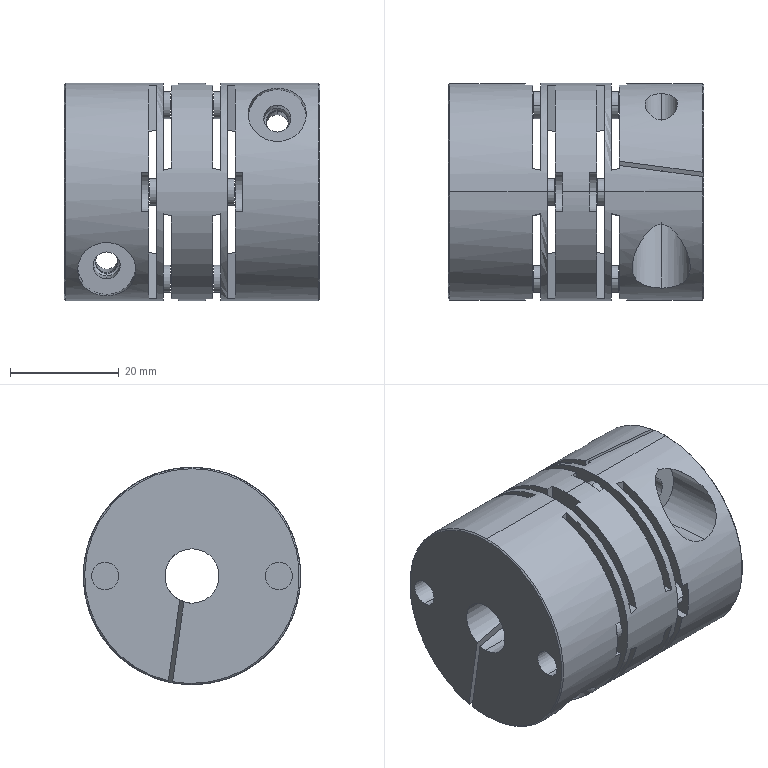Part | STEP file | 0243_Z_MCSLC40-10-16_1 | 1 solid | 159 faces | box 47 x 40 x 40 mm | volume 40763 mm3 | cylinder 78 | plane 67 | cone 14 | commonest cylinder face diameters 5 x28 7.2 x10 24 x10 4.134 x8 6 x4 10.75 x4